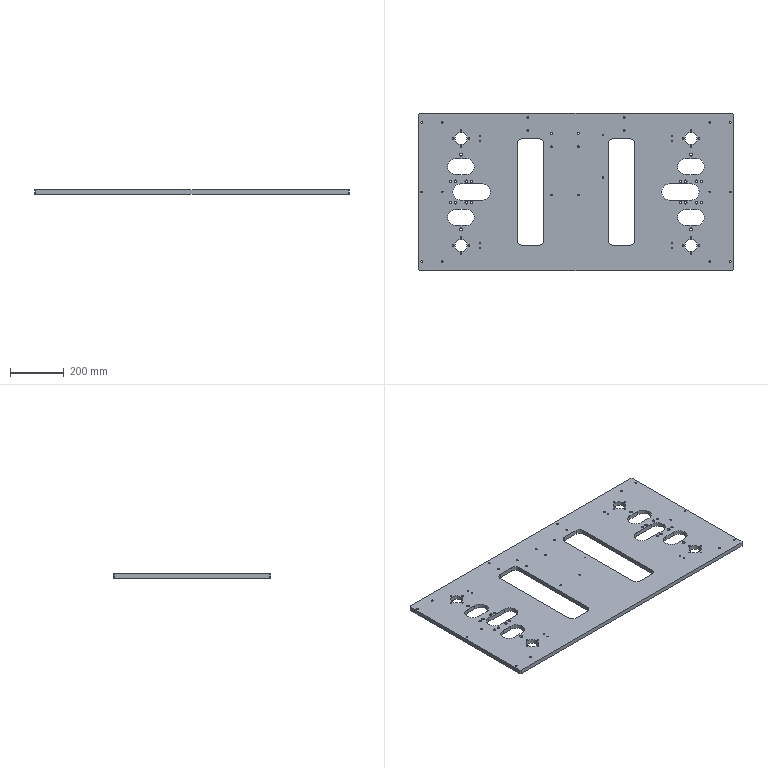Part | SolidWorks | features BaseBody 1 | 1 solid | 200 faces | box 1177 x 588 x 16 mm | volume 9076358 mm3 | cylinder 170 | plane 30 | commonest cylinder face diameters 5 x52 6.8 x44 60 x18 8.5 x16 10 x16 11 x8